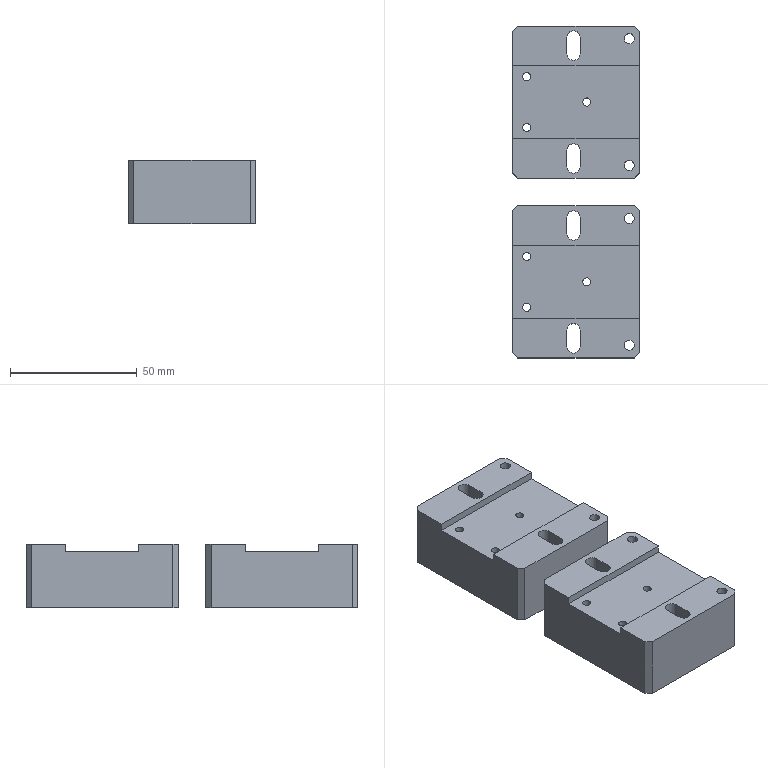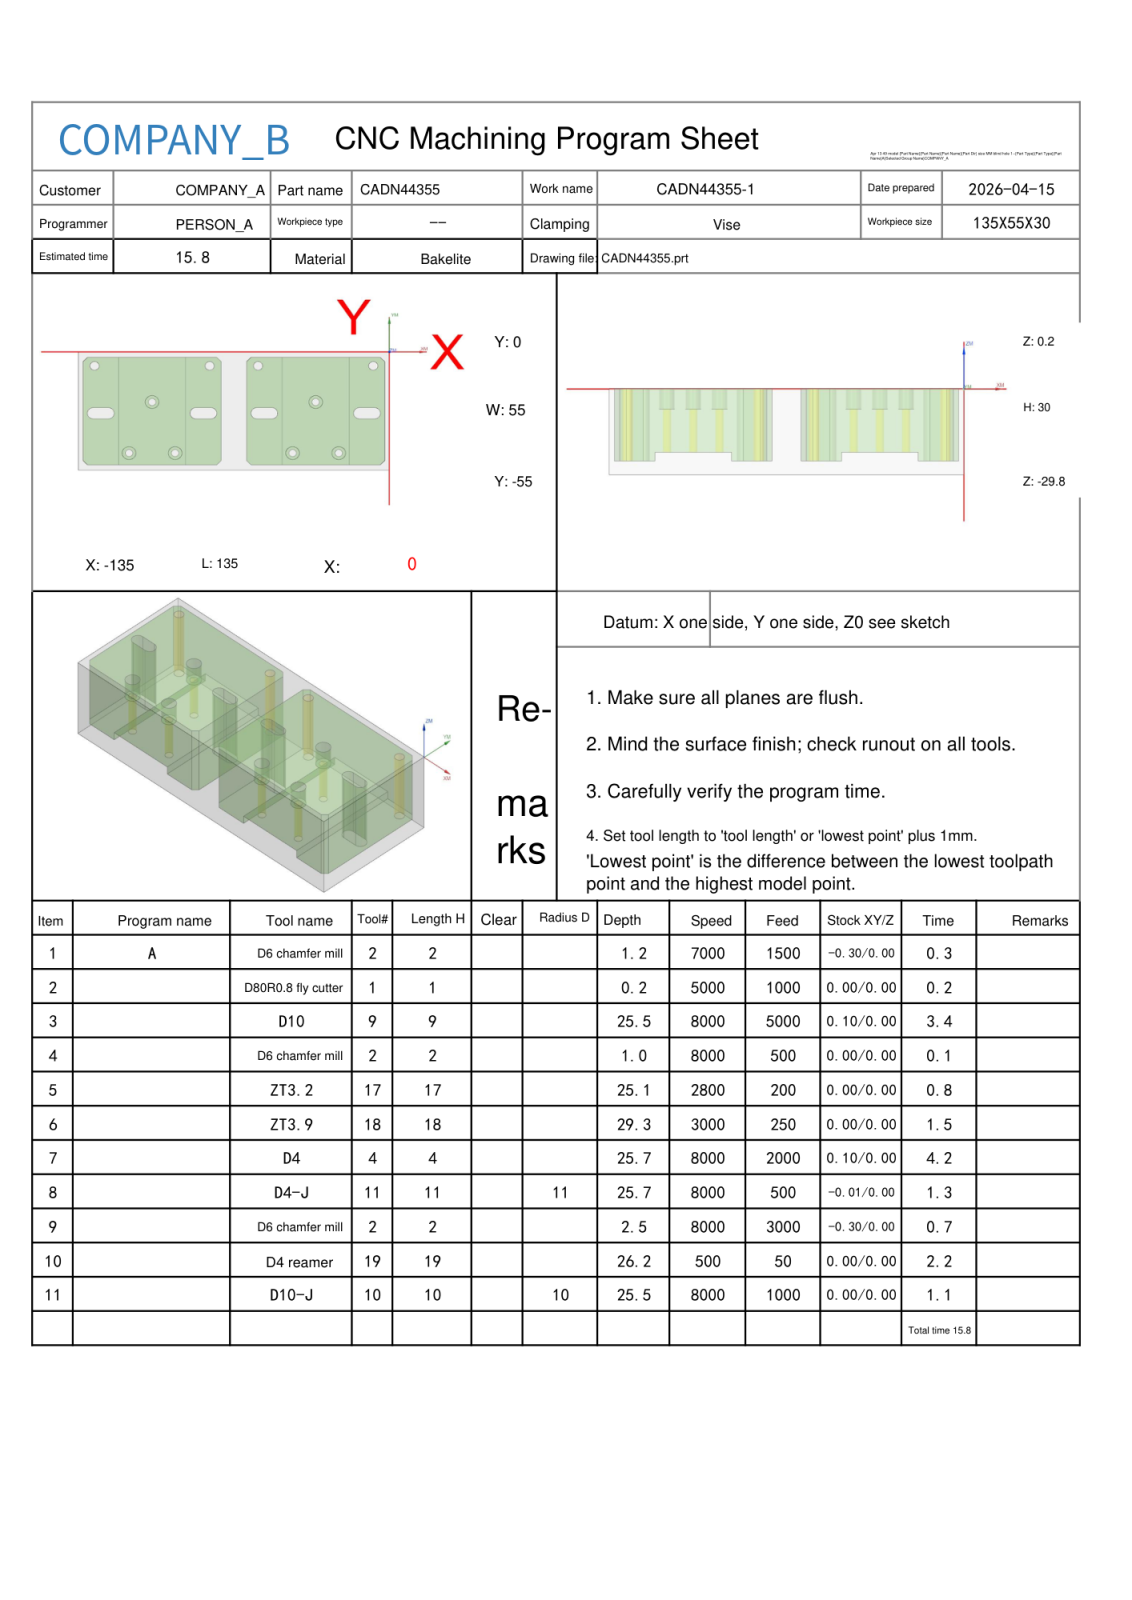NC program | NX | posted by the shop | part box 50 x 131 x 25 mm
Lines 1 to 1279 of 5183, first 1155 of 1277 lines:
%
O0001
(Machine time: 17.84 MIN)
(===Total Tool:9===)
(T2=D6 chamfer mill   D=6.   R=0.   D-  H02 Z=-2.3  )
(T1=D80R0.8 fly cutter D=80.  R=0.8  D-  H01 Z=0.    )
(T9=D10     D=10.  R=0.   D-  H09 Z=-25.3 )
(T17=ZT3.2  D=3.2  DR_a=120 D-  H17 Z=-24.92)
(T18=ZT3.9  D=3.9  DR_a=120 D-  H18 Z=-29.13)
(T4=D4      D=4.   R=0.   D-  H04 Z=-25.5 )
(T11=D4-J   D=4.   R=0.   D11 H11 Z=-25.5 )
(T19=D4 reamer   D=4.   DR_a=180 D-  H19 Z=-26.  )
(T10=D10-J  D=10.  R=0.   D10 H10 Z=-25.3 )
G80 G90 G17 G49 G40
G91 G28 Z0
M01
N1 T02 M06
(D6 chamfer mill  D=6. R=0. H=02 ce=-0.30 di=0.00)
G00 G90 G54 X-1.3 Y-41.546 M03 S7000
G43 H02 Z20.
M08
Z2.5
G01 Y-50.453 Z-.742 F1500.
X-1.338 Y-50.66 Z-.819
X-1.419 Y-50.855 Z-.895
X-1.538 Y-51.028 Z-.972
X-1.593 Y-51.083 Z-1.
X-3.417 Y-52.907
G02 X-4.124 Y-53.2 I-.707 J.707
G01 X-59.876
G02 X-60.583 Y-52.907 I0.0 J1.
G01 X-62.407 Y-51.083
G02 X-62.7 Y-50.376 I.707 J.707
G01 Y-4.624
G02 X-62.407 Y-3.917 I1. J0.0
G01 X-60.583 Y-2.093
G02 X-59.876 Y-1.8 I.707 J-.707
G01 X-4.124
G02 X-3.417 Y-2.093 I0.0 J-1.
G01 X-1.593 Y-3.917
G02 X-1.3 Y-4.624 I-.707 J-.707
G01 Y-50.376
G02 X-1.593 Y-51.083 I-1. J0.0
G01 X-1.946 Y-51.436
Z1.5
G00 Z20.
X-72.3 Y-41.546
Z2.5
G01 Y-50.453 Z-.742
X-72.338 Y-50.66 Z-.819
X-72.419 Y-50.855 Z-.895
X-72.538 Y-51.028 Z-.972
X-72.593 Y-51.083 Z-1.
X-74.417 Y-52.907
G02 X-75.124 Y-53.2 I-.707 J.707
G01 X-130.876
G02 X-131.583 Y-52.907 I0.0 J1.
G01 X-133.407 Y-51.083
G02 X-133.7 Y-50.376 I.707 J.707
G01 Y-4.624
G02 X-133.407 Y-3.917 I1. J0.0
G01 X-131.583 Y-2.093
G02 X-130.876 Y-1.8 I.707 J-.707
G01 X-75.124
G02 X-74.417 Y-2.093 I0.0 J-1.
G01 X-72.593 Y-3.917
G02 X-72.3 Y-4.624 I-.707 J-.707
G01 Y-50.376
G02 X-72.593 Y-51.083 I-1. J0.0
G01 X-72.946 Y-51.436
Z1.5
G00 Z20.
G91 G28 Z0.0
M05
M09
G91 G28 Z0.0
M01
N2 T01 M06
(D80R0.8 fly cutter  D=80. R=0.8 H=01 ce=0.00 di=0.00)
G00 G90 G54 X-178. Y-27.5 M03 S5000
G43 H01 Z20.
M08
Z2.
G01 Z0.0 F1000.
X-173.
X38.
X43.
Z2.
G00 Z20.
G91 G28 Z0.0
M05
M09
G91 G28 Z0.0
M01
N3 T09 M06
(D10  D=10. R=0. H=09 ce=0.10 di=0.00)
G00 G90 G54 X-32. Y-57.6 M03 S8000
G43 H09 Z20.
M08
Z.5
G01 X-60. Z.412 F5000.
G02 X-63.606 Y-56.106 Z.399 I0.0 J5.1
G01 X-65.606 Y-54.106 Z.39
G02 X-67.1 Y-50.5 Z.377 I3.606 J3.606
G01 Y-4.5 Z.232
G02 X-65.606 Y-.894 Z.219 I5.1 J0.0
G01 X-63.606 Y1.106 Z.21
G02 X-60. Y2.6 Z.198 I3.606 J-3.606
G01 X-4. Z.021
G02 X-.394 Y1.106 Z.008 I0.0 J-5.1
G01 X1.606 Y-.894 Z-.001
G02 X3.1 Y-4.5 Z-.014 I-3.606 J-3.606
G01 Y-50.5 Z-.159
G02 X1.606 Y-54.106 Z-.172 I-5.1 J0.0
G01 X-.394 Y-56.106 Z-.181
G02 X-4. Y-57.6 Z-.193 I-3.606 J3.606
G01 X-60. Z-.37
G02 X-63.606 Y-56.106 Z-.383 I0.0 J5.1
G01 X-65.606 Y-54.106 Z-.392
G02 X-67.1 Y-50.5 Z-.405 I3.606 J3.606
G01 Y-4.5 Z-.55
G02 X-65.606 Y-.894 Z-.563 I5.1 J0.0
G01 X-63.606 Y1.106 Z-.572
G02 X-60. Y2.6 Z-.584 I3.606 J-3.606
G01 X-4. Z-.761
G02 X-.394 Y1.106 Z-.774 I0.0 J-5.1
G01 X1.606 Y-.894 Z-.783
G02 X3.1 Y-4.5 Z-.795 I-3.606 J-3.606
G01 Y-50.5 Z-.941
G02 X1.606 Y-54.106 Z-.954 I-5.1 J0.0
G01 X-.394 Y-56.106 Z-.962
G02 X-4. Y-57.6 Z-.975 I-3.606 J3.606
G01 X-60. Z-1.152
G02 X-63.606 Y-56.106 Z-1.165 I0.0 J5.1
G01 X-65.606 Y-54.106 Z-1.174
G02 X-67.1 Y-50.5 Z-1.186 I3.606 J3.606
G01 Y-4.5 Z-1.332
G02 X-65.606 Y-.894 Z-1.344 I5.1 J0.0
G01 X-63.606 Y1.106 Z-1.353
G02 X-60. Y2.6 Z-1.366 I3.606 J-3.606
G01 X-4. Z-1.543
G02 X-.394 Y1.106 Z-1.556 I0.0 J-5.1
G01 X1.606 Y-.894 Z-1.565
G02 X3.1 Y-4.5 Z-1.577 I-3.606 J-3.606
G01 Y-50.5 Z-1.723
G02 X1.606 Y-54.106 Z-1.735 I-5.1 J0.0
G01 X-.394 Y-56.106 Z-1.744
G02 X-4. Y-57.6 Z-1.757 I-3.606 J3.606
G01 X-60. Z-1.934
G02 X-63.606 Y-56.106 Z-1.947 I0.0 J5.1
G01 X-65.606 Y-54.106 Z-1.956
G02 X-67.1 Y-50.5 Z-1.968 I3.606 J3.606
G01 Y-4.5 Z-2.114
G02 X-65.606 Y-.894 Z-2.126 I5.1 J0.0
G01 X-63.606 Y1.106 Z-2.135
G02 X-60. Y2.6 Z-2.148 I3.606 J-3.606
G01 X-4. Z-2.325
G02 X-.394 Y1.106 Z-2.338 I0.0 J-5.1
G01 X1.606 Y-.894 Z-2.346
G02 X3.1 Y-4.5 Z-2.359 I-3.606 J-3.606
G01 Y-50.5 Z-2.505
G02 X1.606 Y-54.106 Z-2.517 I-5.1 J0.0
G01 X-.394 Y-56.106 Z-2.526
G02 X-4. Y-57.6 Z-2.539 I-3.606 J3.606
G01 X-60. Z-2.716
G02 X-63.606 Y-56.106 Z-2.728 I0.0 J5.1
G01 X-65.606 Y-54.106 Z-2.737
G02 X-67.1 Y-50.5 Z-2.75 I3.606 J3.606
G01 Y-4.5 Z-2.895
G02 X-65.606 Y-.894 Z-2.908 I5.1 J0.0
G01 X-63.606 Y1.106 Z-2.917
G02 X-60. Y2.6 Z-2.93 I3.606 J-3.606
G01 X-4. Z-3.107
G02 X-.394 Y1.106 Z-3.119 I0.0 J-5.1
G01 X1.606 Y-.894 Z-3.128
G02 X3.1 Y-4.5 Z-3.141 I-3.606 J-3.606
G01 Y-50.5 Z-3.286
G02 X1.606 Y-54.106 Z-3.299 I-5.1 J0.0
G01 X-.394 Y-56.106 Z-3.308
G02 X-4. Y-57.6 Z-3.321 I-3.606 J3.606
G01 X-60. Z-3.498
G02 X-63.606 Y-56.106 Z-3.51 I0.0 J5.1
G01 X-65.606 Y-54.106 Z-3.519
G02 X-67.1 Y-50.5 Z-3.532 I3.606 J3.606
G01 Y-4.5 Z-3.677
G02 X-65.606 Y-.894 Z-3.69 I5.1 J0.0
G01 X-63.606 Y1.106 Z-3.699
G02 X-60. Y2.6 Z-3.712 I3.606 J-3.606
G01 X-4. Z-3.888
G02 X-.394 Y1.106 Z-3.901 I0.0 J-5.1
G01 X1.606 Y-.894 Z-3.91
G02 X3.1 Y-4.5 Z-3.923 I-3.606 J-3.606
G01 Y-50.5 Z-4.068
G02 X1.606 Y-54.106 Z-4.081 I-5.1 J0.0
G01 X-.394 Y-56.106 Z-4.09
G02 X-4. Y-57.6 Z-4.102 I-3.606 J3.606
G01 X-60. Z-4.279
G02 X-63.606 Y-56.106 Z-4.292 I0.0 J5.1
G01 X-65.606 Y-54.106 Z-4.301
G02 X-67.1 Y-50.5 Z-4.314 I3.606 J3.606
G01 Y-4.5 Z-4.459
G02 X-65.606 Y-.894 Z-4.472 I5.1 J0.0
G01 X-63.606 Y1.106 Z-4.481
G02 X-60. Y2.6 Z-4.493 I3.606 J-3.606
G01 X-4. Z-4.67
G02 X-.394 Y1.106 Z-4.683 I0.0 J-5.1
G01 X1.606 Y-.894 Z-4.692
G02 X3.1 Y-4.5 Z-4.705 I-3.606 J-3.606
G01 Y-50.5 Z-4.85
G02 X1.606 Y-54.106 Z-4.863 I-5.1 J0.0
G01 X-.394 Y-56.106 Z-4.872
G02 X-4. Y-57.6 Z-4.884 I-3.606 J3.606
G01 X-60. Z-5.061
G02 X-63.606 Y-56.106 Z-5.074 I0.0 J5.1
G01 X-65.606 Y-54.106 Z-5.083
G02 X-67.1 Y-50.5 Z-5.095 I3.606 J3.606
G01 Y-4.5 Z-5.241
G02 X-65.606 Y-.894 Z-5.254 I5.1 J0.0
G01 X-63.606 Y1.106 Z-5.262
G02 X-60. Y2.6 Z-5.275 I3.606 J-3.606
G01 X-4. Z-5.452
G02 X-.394 Y1.106 Z-5.465 I0.0 J-5.1
G01 X1.606 Y-.894 Z-5.474
G02 X3.1 Y-4.5 Z-5.486 I-3.606 J-3.606
G01 Y-50.5 Z-5.632
G02 X1.606 Y-54.106 Z-5.644 I-5.1 J0.0
G01 X-.394 Y-56.106 Z-5.653
G02 X-4. Y-57.6 Z-5.666 I-3.606 J3.606
G01 X-60. Z-5.843
G02 X-63.606 Y-56.106 Z-5.856 I0.0 J5.1
G01 X-65.606 Y-54.106 Z-5.865
G02 X-67.1 Y-50.5 Z-5.877 I3.606 J3.606
G01 Y-4.5 Z-6.023
G02 X-65.606 Y-.894 Z-6.035 I5.1 J0.0
G01 X-63.606 Y1.106 Z-6.044
G02 X-60. Y2.6 Z-6.057 I3.606 J-3.606
G01 X-4. Z-6.234
G02 X-.394 Y1.106 Z-6.247 I0.0 J-5.1
G01 X1.606 Y-.894 Z-6.256
G02 X3.1 Y-4.5 Z-6.268 I-3.606 J-3.606
G01 Y-50.5 Z-6.414
G02 X1.606 Y-54.106 Z-6.426 I-5.1 J0.0
G01 X-.394 Y-56.106 Z-6.435
G02 X-4. Y-57.6 Z-6.448 I-3.606 J3.606
G01 X-60. Z-6.625
G02 X-63.606 Y-56.106 Z-6.638 I0.0 J5.1
G01 X-65.606 Y-54.106 Z-6.646
G02 X-67.1 Y-50.5 Z-6.659 I3.606 J3.606
G01 Y-4.5 Z-6.805
G02 X-65.606 Y-.894 Z-6.817 I5.1 J0.0
G01 X-63.606 Y1.106 Z-6.826
G02 X-60. Y2.6 Z-6.839 I3.606 J-3.606
G01 X-4. Z-7.016
G02 X-.394 Y1.106 Z-7.028 I0.0 J-5.1
G01 X1.606 Y-.894 Z-7.037
G02 X3.1 Y-4.5 Z-7.05 I-3.606 J-3.606
G01 Y-50.5 Z-7.195
G02 X1.606 Y-54.106 Z-7.208 I-5.1 J0.0
G01 X-.394 Y-56.106 Z-7.217
G02 X-4. Y-57.6 Z-7.23 I-3.606 J3.606
G01 X-60. Z-7.407
G02 X-63.606 Y-56.106 Z-7.419 I0.0 J5.1
G01 X-65.606 Y-54.106 Z-7.428
G02 X-67.1 Y-50.5 Z-7.441 I3.606 J3.606
G01 Y-4.5 Z-7.586
G02 X-65.606 Y-.894 Z-7.599 I5.1 J0.0
G01 X-63.606 Y1.106 Z-7.608
G02 X-60. Y2.6 Z-7.621 I3.606 J-3.606
G01 X-4. Z-7.798
G02 X-.394 Y1.106 Z-7.81 I0.0 J-5.1
G01 X1.606 Y-.894 Z-7.819
G02 X3.1 Y-4.5 Z-7.832 I-3.606 J-3.606
G01 Y-50.5 Z-7.977
G02 X1.606 Y-54.106 Z-7.99 I-5.1 J0.0
G01 X-.394 Y-56.106 Z-7.999
G02 X-4. Y-57.6 Z-8.012 I-3.606 J3.606
G01 X-60. Z-8.188
G02 X-63.606 Y-56.106 Z-8.201 I0.0 J5.1
G01 X-65.606 Y-54.106 Z-8.21
G02 X-67.1 Y-50.5 Z-8.223 I3.606 J3.606
G01 Y-4.5 Z-8.368
G02 X-65.606 Y-.894 Z-8.381 I5.1 J0.0
G01 X-63.606 Y1.106 Z-8.39
G02 X-60. Y2.6 Z-8.402 I3.606 J-3.606
G01 X-4. Z-8.579
G02 X-.394 Y1.106 Z-8.592 I0.0 J-5.1
G01 X1.606 Y-.894 Z-8.601
G02 X3.1 Y-4.5 Z-8.614 I-3.606 J-3.606
G01 Y-50.5 Z-8.759
G02 X1.606 Y-54.106 Z-8.772 I-5.1 J0.0
G01 X-.394 Y-56.106 Z-8.781
G02 X-4. Y-57.6 Z-8.793 I-3.606 J3.606
G01 X-60. Z-8.97
G02 X-63.606 Y-56.106 Z-8.983 I0.0 J5.1
G01 X-65.606 Y-54.106 Z-8.992
G02 X-67.1 Y-50.5 Z-9.005 I3.606 J3.606
G01 Y-4.5 Z-9.15
G02 X-65.606 Y-.894 Z-9.163 I5.1 J0.0
G01 X-63.606 Y1.106 Z-9.172
G02 X-60. Y2.6 Z-9.184 I3.606 J-3.606
G01 X-4. Z-9.361
G02 X-.394 Y1.106 Z-9.374 I0.0 J-5.1
G01 X1.606 Y-.894 Z-9.383
G02 X3.1 Y-4.5 Z-9.395 I-3.606 J-3.606
G01 Y-50.5 Z-9.541
G02 X1.606 Y-54.106 Z-9.554 I-5.1 J0.0
G01 X-.394 Y-56.106 Z-9.562
G02 X-4. Y-57.6 Z-9.575 I-3.606 J3.606
G01 X-60. Z-9.752
G02 X-63.606 Y-56.106 Z-9.765 I0.0 J5.1
G01 X-65.606 Y-54.106 Z-9.774
G02 X-67.1 Y-50.5 Z-9.786 I3.606 J3.606
G01 Y-4.5 Z-9.932
G02 X-65.606 Y-.894 Z-9.944 I5.1 J0.0
G01 X-63.606 Y1.106 Z-9.953
G02 X-60. Y2.6 Z-9.966 I3.606 J-3.606
G01 X-4. Z-10.143
G02 X-.394 Y1.106 Z-10.156 I0.0 J-5.1
G01 X1.606 Y-.894 Z-10.165
G02 X3.1 Y-4.5 Z-10.177 I-3.606 J-3.606
G01 Y-50.5 Z-10.323
G02 X1.606 Y-54.106 Z-10.335 I-5.1 J0.0
G01 X-.394 Y-56.106 Z-10.344
G02 X-4. Y-57.6 Z-10.357 I-3.606 J3.606
G01 X-60. Z-10.534
G02 X-63.606 Y-56.106 Z-10.547 I0.0 J5.1
G01 X-65.606 Y-54.106 Z-10.556
G02 X-67.1 Y-50.5 Z-10.568 I3.606 J3.606
G01 Y-4.5 Z-10.714
G02 X-65.606 Y-.894 Z-10.726 I5.1 J0.0
G01 X-63.606 Y1.106 Z-10.735
G02 X-60. Y2.6 Z-10.748 I3.606 J-3.606
G01 X-4. Z-10.925
G02 X-.394 Y1.106 Z-10.938 I0.0 J-5.1
G01 X1.606 Y-.894 Z-10.946
G02 X3.1 Y-4.5 Z-10.959 I-3.606 J-3.606
G01 Y-50.5 Z-11.105
G02 X1.606 Y-54.106 Z-11.117 I-5.1 J0.0
G01 X-.394 Y-56.106 Z-11.126
G02 X-4. Y-57.6 Z-11.139 I-3.606 J3.606
G01 X-60. Z-11.316
G02 X-63.606 Y-56.106 Z-11.328 I0.0 J5.1
G01 X-65.606 Y-54.106 Z-11.337
G02 X-67.1 Y-50.5 Z-11.35 I3.606 J3.606
G01 Y-4.5 Z-11.495
G02 X-65.606 Y-.894 Z-11.508 I5.1 J0.0
G01 X-63.606 Y1.106 Z-11.517
G02 X-60. Y2.6 Z-11.53 I3.606 J-3.606
G01 X-4. Z-11.707
G02 X-.394 Y1.106 Z-11.719 I0.0 J-5.1
G01 X1.606 Y-.894 Z-11.728
G02 X3.1 Y-4.5 Z-11.741 I-3.606 J-3.606
G01 Y-50.5 Z-11.886
G02 X1.606 Y-54.106 Z-11.899 I-5.1 J0.0
G01 X-.394 Y-56.106 Z-11.908
G02 X-4. Y-57.6 Z-11.921 I-3.606 J3.606
G01 X-60. Z-12.098
G02 X-63.606 Y-56.106 Z-12.11 I0.0 J5.1
G01 X-65.606 Y-54.106 Z-12.119
G02 X-67.1 Y-50.5 Z-12.132 I3.606 J3.606
G01 Y-4.5 Z-12.277
G02 X-65.606 Y-.894 Z-12.29 I5.1 J0.0
G01 X-63.606 Y1.106 Z-12.299
G02 X-60. Y2.6 Z-12.312 I3.606 J-3.606
G01 X-4. Z-12.488
G02 X-.394 Y1.106 Z-12.501 I0.0 J-5.1
G01 X1.606 Y-.894 Z-12.51
G02 X3.1 Y-4.5 Z-12.523 I-3.606 J-3.606
G01 Y-50.5 Z-12.668
G02 X1.606 Y-54.106 Z-12.681 I-5.1 J0.0
G01 X-.394 Y-56.106 Z-12.69
G02 X-4. Y-57.6 Z-12.702 I-3.606 J3.606
G01 X-60. Z-12.879
G02 X-63.606 Y-56.106 Z-12.892 I0.0 J5.1
G01 X-65.606 Y-54.106 Z-12.901
G02 X-67.1 Y-50.5 Z-12.914 I3.606 J3.606
G01 Y-4.5 Z-13.059
G02 X-65.606 Y-.894 Z-13.072 I5.1 J0.0
G01 X-63.606 Y1.106 Z-13.081
G02 X-60. Y2.6 Z-13.093 I3.606 J-3.606
G01 X-4. Z-13.27
G02 X-.394 Y1.106 Z-13.283 I0.0 J-5.1
G01 X1.606 Y-.894 Z-13.292
G02 X3.1 Y-4.5 Z-13.305 I-3.606 J-3.606
G01 Y-50.5 Z-13.45
G02 X1.606 Y-54.106 Z-13.463 I-5.1 J0.0
G01 X-.394 Y-56.106 Z-13.472
G02 X-4. Y-57.6 Z-13.484 I-3.606 J3.606
G01 X-60. Z-13.661
G02 X-63.606 Y-56.106 Z-13.674 I0.0 J5.1
G01 X-65.606 Y-54.106 Z-13.683
G02 X-67.1 Y-50.5 Z-13.695 I3.606 J3.606
G01 Y-4.5 Z-13.841
G02 X-65.606 Y-.894 Z-13.854 I5.1 J0.0
G01 X-63.606 Y1.106 Z-13.862
G02 X-60. Y2.6 Z-13.875 I3.606 J-3.606
G01 X-4. Z-14.052
G02 X-.394 Y1.106 Z-14.065 I0.0 J-5.1
G01 X1.606 Y-.894 Z-14.074
G02 X3.1 Y-4.5 Z-14.086 I-3.606 J-3.606
G01 Y-50.5 Z-14.232
G02 X1.606 Y-54.106 Z-14.244 I-5.1 J0.0
G01 X-.394 Y-56.106 Z-14.253
G02 X-4. Y-57.6 Z-14.266 I-3.606 J3.606
G01 X-60. Z-14.443
G02 X-63.606 Y-56.106 Z-14.456 I0.0 J5.1
G01 X-65.606 Y-54.106 Z-14.465
G02 X-67.1 Y-50.5 Z-14.477 I3.606 J3.606
G01 Y-4.5 Z-14.623
G02 X-65.606 Y-.894 Z-14.635 I5.1 J0.0
G01 X-63.606 Y1.106 Z-14.644
G02 X-60. Y2.6 Z-14.657 I3.606 J-3.606
G01 X-4. Z-14.834
G02 X-.394 Y1.106 Z-14.847 I0.0 J-5.1
G01 X1.606 Y-.894 Z-14.856
G02 X3.1 Y-4.5 Z-14.868 I-3.606 J-3.606
G01 Y-50.5 Z-15.014
G02 X1.606 Y-54.106 Z-15.026 I-5.1 J0.0
G01 X-.394 Y-56.106 Z-15.035
G02 X-4. Y-57.6 Z-15.048 I-3.606 J3.606
G01 X-60. Z-15.225
G02 X-63.606 Y-56.106 Z-15.238 I0.0 J5.1
G01 X-65.606 Y-54.106 Z-15.246
G02 X-67.1 Y-50.5 Z-15.259 I3.606 J3.606
G01 Y-4.5 Z-15.405
G02 X-65.606 Y-.894 Z-15.417 I5.1 J0.0
G01 X-63.606 Y1.106 Z-15.426
G02 X-60. Y2.6 Z-15.439 I3.606 J-3.606
G01 X-4. Z-15.616
G02 X-.394 Y1.106 Z-15.628 I0.0 J-5.1
G01 X1.606 Y-.894 Z-15.637
G02 X3.1 Y-4.5 Z-15.65 I-3.606 J-3.606
G01 Y-50.5 Z-15.795
G02 X1.606 Y-54.106 Z-15.808 I-5.1 J0.0
G01 X-.394 Y-56.106 Z-15.817
G02 X-4. Y-57.6 Z-15.83 I-3.606 J3.606
G01 X-60. Z-16.007
G02 X-63.606 Y-56.106 Z-16.019 I0.0 J5.1
G01 X-65.606 Y-54.106 Z-16.028
G02 X-67.1 Y-50.5 Z-16.041 I3.606 J3.606
G01 Y-4.5 Z-16.186
G02 X-65.606 Y-.894 Z-16.199 I5.1 J0.0
G01 X-63.606 Y1.106 Z-16.208
G02 X-60. Y2.6 Z-16.221 I3.606 J-3.606
G01 X-4. Z-16.398
G02 X-.394 Y1.106 Z-16.41 I0.0 J-5.1
G01 X1.606 Y-.894 Z-16.419
G02 X3.1 Y-4.5 Z-16.432 I-3.606 J-3.606
G01 Y-50.5 Z-16.577
G02 X1.606 Y-54.106 Z-16.59 I-5.1 J0.0
G01 X-.394 Y-56.106 Z-16.599
G02 X-4. Y-57.6 Z-16.612 I-3.606 J3.606
G01 X-60. Z-16.788
G02 X-63.606 Y-56.106 Z-16.801 I0.0 J5.1
G01 X-65.606 Y-54.106 Z-16.81
G02 X-67.1 Y-50.5 Z-16.823 I3.606 J3.606
G01 Y-4.5 Z-16.968
G02 X-65.606 Y-.894 Z-16.981 I5.1 J0.0
G01 X-63.606 Y1.106 Z-16.99
G02 X-60. Y2.6 Z-17.002 I3.606 J-3.606
G01 X-4. Z-17.179
G02 X-.394 Y1.106 Z-17.192 I0.0 J-5.1
G01 X1.606 Y-.894 Z-17.201
G02 X3.1 Y-4.5 Z-17.214 I-3.606 J-3.606
G01 Y-50.5 Z-17.359
G02 X1.606 Y-54.106 Z-17.372 I-5.1 J0.0
G01 X-.394 Y-56.106 Z-17.381
G02 X-4. Y-57.6 Z-17.393 I-3.606 J3.606
G01 X-60. Z-17.57
G02 X-63.606 Y-56.106 Z-17.583 I0.0 J5.1
G01 X-65.606 Y-54.106 Z-17.592
G02 X-67.1 Y-50.5 Z-17.605 I3.606 J3.606
G01 Y-4.5 Z-17.75
G02 X-65.606 Y-.894 Z-17.763 I5.1 J0.0
G01 X-63.606 Y1.106 Z-17.772
G02 X-60. Y2.6 Z-17.784 I3.606 J-3.606
G01 X-4. Z-17.961
G02 X-.394 Y1.106 Z-17.974 I0.0 J-5.1
G01 X1.606 Y-.894 Z-17.983
G02 X3.1 Y-4.5 Z-17.995 I-3.606 J-3.606
G01 Y-50.5 Z-18.141
G02 X1.606 Y-54.106 Z-18.154 I-5.1 J0.0
G01 X-.394 Y-56.106 Z-18.162
G02 X-4. Y-57.6 Z-18.175 I-3.606 J3.606
G01 X-60. Z-18.352
G02 X-63.606 Y-56.106 Z-18.365 I0.0 J5.1
G01 X-65.606 Y-54.106 Z-18.374
G02 X-67.1 Y-50.5 Z-18.386 I3.606 J3.606
G01 Y-4.5 Z-18.532
G02 X-65.606 Y-.894 Z-18.544 I5.1 J0.0
G01 X-63.606 Y1.106 Z-18.553
G02 X-60. Y2.6 Z-18.566 I3.606 J-3.606
G01 X-4. Z-18.743
G02 X-.394 Y1.106 Z-18.756 I0.0 J-5.1
G01 X1.606 Y-.894 Z-18.765
G02 X3.1 Y-4.5 Z-18.777 I-3.606 J-3.606
G01 Y-50.5 Z-18.923
G02 X1.606 Y-54.106 Z-18.935 I-5.1 J0.0
G01 X-.394 Y-56.106 Z-18.944
G02 X-4. Y-57.6 Z-18.957 I-3.606 J3.606
G01 X-60. Z-19.134
G02 X-63.606 Y-56.106 Z-19.147 I0.0 J5.1
G01 X-65.606 Y-54.106 Z-19.156
G02 X-67.1 Y-50.5 Z-19.168 I3.606 J3.606
G01 Y-4.5 Z-19.314
G02 X-65.606 Y-.894 Z-19.326 I5.1 J0.0
G01 X-63.606 Y1.106 Z-19.335
G02 X-60. Y2.6 Z-19.348 I3.606 J-3.606
G01 X-4. Z-19.525
G02 X-.394 Y1.106 Z-19.538 I0.0 J-5.1
G01 X1.606 Y-.894 Z-19.546
G02 X3.1 Y-4.5 Z-19.559 I-3.606 J-3.606
G01 Y-50.5 Z-19.705
G02 X1.606 Y-54.106 Z-19.717 I-5.1 J0.0
G01 X-.394 Y-56.106 Z-19.726
G02 X-4. Y-57.6 Z-19.739 I-3.606 J3.606
G01 X-60. Z-19.916
G02 X-63.606 Y-56.106 Z-19.928 I0.0 J5.1
G01 X-65.606 Y-54.106 Z-19.937
G02 X-67.1 Y-50.5 Z-19.95 I3.606 J3.606
G01 Y-4.5 Z-20.095
G02 X-65.606 Y-.894 Z-20.108 I5.1 J0.0
G01 X-63.606 Y1.106 Z-20.117
G02 X-60. Y2.6 Z-20.13 I3.606 J-3.606
G01 X-4. Z-20.307
G02 X-.394 Y1.106 Z-20.319 I0.0 J-5.1
G01 X1.606 Y-.894 Z-20.328
G02 X3.1 Y-4.5 Z-20.341 I-3.606 J-3.606
G01 Y-50.5 Z-20.486
G02 X1.606 Y-54.106 Z-20.499 I-5.1 J0.0
G01 X-.394 Y-56.106 Z-20.508
G02 X-4. Y-57.6 Z-20.521 I-3.606 J3.606
G01 X-60. Z-20.698
G02 X-63.606 Y-56.106 Z-20.71 I0.0 J5.1
G01 X-65.606 Y-54.106 Z-20.719
G02 X-67.1 Y-50.5 Z-20.732 I3.606 J3.606
G01 Y-4.5 Z-20.877
G02 X-65.606 Y-.894 Z-20.89 I5.1 J0.0
G01 X-63.606 Y1.106 Z-20.899
G02 X-60. Y2.6 Z-20.912 I3.606 J-3.606
G01 X-4. Z-21.088
G02 X-.394 Y1.106 Z-21.101 I0.0 J-5.1
G01 X1.606 Y-.894 Z-21.11
G02 X3.1 Y-4.5 Z-21.123 I-3.606 J-3.606
G01 Y-50.5 Z-21.268
G02 X1.606 Y-54.106 Z-21.281 I-5.1 J0.0
G01 X-.394 Y-56.106 Z-21.29
G02 X-4. Y-57.6 Z-21.302 I-3.606 J3.606
G01 X-60. Z-21.479
G02 X-63.606 Y-56.106 Z-21.492 I0.0 J5.1
G01 X-65.606 Y-54.106 Z-21.501
G02 X-67.1 Y-50.5 Z-21.514 I3.606 J3.606
G01 Y-4.5 Z-21.659
G02 X-65.606 Y-.894 Z-21.672 I5.1 J0.0
G01 X-63.606 Y1.106 Z-21.681
G02 X-60. Y2.6 Z-21.693 I3.606 J-3.606
G01 X-4. Z-21.87
G02 X-.394 Y1.106 Z-21.883 I0.0 J-5.1
G01 X1.606 Y-.894 Z-21.892
G02 X3.1 Y-4.5 Z-21.905 I-3.606 J-3.606
G01 Y-50.5 Z-22.05
G02 X1.606 Y-54.106 Z-22.063 I-5.1 J0.0
G01 X-.394 Y-56.106 Z-22.072
G02 X-4. Y-57.6 Z-22.084 I-3.606 J3.606
G01 X-60. Z-22.261
G02 X-63.606 Y-56.106 Z-22.274 I0.0 J5.1
G01 X-65.606 Y-54.106 Z-22.283
G02 X-67.1 Y-50.5 Z-22.295 I3.606 J3.606
G01 Y-4.5 Z-22.441
G02 X-65.606 Y-.894 Z-22.454 I5.1 J0.0
G01 X-63.606 Y1.106 Z-22.462
G02 X-60. Y2.6 Z-22.475 I3.606 J-3.606
G01 X-4. Z-22.652
G02 X-.394 Y1.106 Z-22.665 I0.0 J-5.1
G01 X1.606 Y-.894 Z-22.674
G02 X3.1 Y-4.5 Z-22.686 I-3.606 J-3.606
G01 Y-50.5 Z-22.832
G02 X1.606 Y-54.106 Z-22.844 I-5.1 J0.0
G01 X-.394 Y-56.106 Z-22.853
G02 X-4. Y-57.6 Z-22.866 I-3.606 J3.606
G01 X-60. Z-23.043
G02 X-63.606 Y-56.106 Z-23.056 I0.0 J5.1
G01 X-65.606 Y-54.106 Z-23.065
G02 X-67.1 Y-50.5 Z-23.077 I3.606 J3.606
G01 Y-4.5 Z-23.223
G02 X-65.606 Y-.894 Z-23.235 I5.1 J0.0
G01 X-63.606 Y1.106 Z-23.244
G02 X-60. Y2.6 Z-23.257 I3.606 J-3.606
G01 X-4. Z-23.434
G02 X-.394 Y1.106 Z-23.447 I0.0 J-5.1
G01 X1.606 Y-.894 Z-23.456
G02 X3.1 Y-4.5 Z-23.468 I-3.606 J-3.606
G01 Y-50.5 Z-23.614
G02 X1.606 Y-54.106 Z-23.626 I-5.1 J0.0
G01 X-.394 Y-56.106 Z-23.635
G02 X-4. Y-57.6 Z-23.648 I-3.606 J3.606
G01 X-60. Z-23.825
G02 X-63.606 Y-56.106 Z-23.838 I0.0 J5.1
G01 X-65.606 Y-54.106 Z-23.846
G02 X-67.1 Y-50.5 Z-23.859 I3.606 J3.606
G01 Y-4.5 Z-24.005
G02 X-65.606 Y-.894 Z-24.017 I5.1 J0.0
G01 X-63.606 Y1.106 Z-24.026
G02 X-60. Y2.6 Z-24.039 I3.606 J-3.606
G01 X-4. Z-24.216
G02 X-.394 Y1.106 Z-24.228 I0.0 J-5.1
G01 X1.606 Y-.894 Z-24.237
G02 X3.1 Y-4.5 Z-24.25 I-3.606 J-3.606
G01 Y-50.5 Z-24.395
G02 X1.606 Y-54.106 Z-24.408 I-5.1 J0.0
G01 X-.394 Y-56.106 Z-24.417
G02 X-4. Y-57.6 Z-24.43 I-3.606 J3.606
G01 X-60. Z-24.607
G02 X-63.606 Y-56.106 Z-24.619 I0.0 J5.1
G01 X-65.606 Y-54.106 Z-24.628
G02 X-67.1 Y-50.5 Z-24.641 I3.606 J3.606
G01 Y-4.5 Z-24.786
G02 X-65.606 Y-.894 Z-24.799 I5.1 J0.0
G01 X-63.606 Y1.106 Z-24.808
G02 X-60. Y2.6 Z-24.821 I3.606 J-3.606
G01 X-4. Z-24.998
G02 X-.394 Y1.106 Z-25.01 I0.0 J-5.1
G01 X1.606 Y-.894 Z-25.019
G02 X3.1 Y-4.5 Z-25.032 I-3.606 J-3.606
G01 Y-50.5 Z-25.177
G02 X1.606 Y-54.106 Z-25.19 I-5.1 J0.0
G01 X-.394 Y-56.106 Z-25.199
G02 X-4. Y-57.6 Z-25.212 I-3.606 J3.606
G01 X-32. Z-25.3
X-60.
G02 X-63.606 Y-56.106 I0.0 J5.1
G01 X-65.606 Y-54.106
G02 X-67.1 Y-50.5 I3.606 J3.606
G01 Y-4.5
G02 X-65.606 Y-.894 I5.1 J0.0
G01 X-63.606 Y1.106
G02 X-60. Y2.6 I3.606 J-3.606
G01 X-4.
G02 X-.394 Y1.106 I0.0 J-5.1
G01 X1.606 Y-.894
G02 X3.1 Y-4.5 I-3.606 J-3.606
G01 Y-50.5
G02 X1.606 Y-54.106 I-5.1 J0.0
G01 X-.394 Y-56.106
G02 X-4. Y-57.6 I-3.606 J3.606
G01 X-32.
X-32.5
Z-24.3
G00 Z20.
X-103.
Z.5
G01 X-131. Z.412
G02 X-134.606 Y-56.106 Z.399 I0.0 J5.1
G01 X-136.606 Y-54.106 Z.39
G02 X-138.1 Y-50.5 Z.377 I3.606 J3.606
G01 Y-4.5 Z.232
G02 X-136.606 Y-.894 Z.219 I5.1 J0.0
G01 X-134.606 Y1.106 Z.21
G02 X-131. Y2.6 Z.198 I3.606 J-3.606
G01 X-75. Z.021
G02 X-71.394 Y1.106 Z.008 I0.0 J-5.1
G01 X-69.394 Y-.894 Z-.001
G02 X-67.9 Y-4.5 Z-.014 I-3.606 J-3.606
G01 Y-50.5 Z-.159
G02 X-69.394 Y-54.106 Z-.172 I-5.1 J0.0
G01 X-71.394 Y-56.106 Z-.181
G02 X-75. Y-57.6 Z-.193 I-3.606 J3.606
G01 X-131. Z-.37
G02 X-134.606 Y-56.106 Z-.383 I0.0 J5.1
G01 X-136.606 Y-54.106 Z-.392
G02 X-138.1 Y-50.5 Z-.405 I3.606 J3.606
G01 Y-4.5 Z-.55
G02 X-136.606 Y-.894 Z-.563 I5.1 J0.0
G01 X-134.606 Y1.106 Z-.572
G02 X-131. Y2.6 Z-.584 I3.606 J-3.606
G01 X-75. Z-.761
G02 X-71.394 Y1.106 Z-.774 I0.0 J-5.1
G01 X-69.394 Y-.894 Z-.783
G02 X-67.9 Y-4.5 Z-.795 I-3.606 J-3.606
G01 Y-50.5 Z-.941
G02 X-69.394 Y-54.106 Z-.954 I-5.1 J0.0
G01 X-71.394 Y-56.106 Z-.962
G02 X-75. Y-57.6 Z-.975 I-3.606 J3.606
G01 X-131. Z-1.152
G02 X-134.606 Y-56.106 Z-1.165 I0.0 J5.1
G01 X-136.606 Y-54.106 Z-1.174
G02 X-138.1 Y-50.5 Z-1.186 I3.606 J3.606
G01 Y-4.5 Z-1.332
G02 X-136.606 Y-.894 Z-1.344 I5.1 J0.0
G01 X-134.606 Y1.106 Z-1.353
G02 X-131. Y2.6 Z-1.366 I3.606 J-3.606
G01 X-75. Z-1.543
G02 X-71.394 Y1.106 Z-1.556 I0.0 J-5.1
G01 X-69.394 Y-.894 Z-1.565
G02 X-67.9 Y-4.5 Z-1.577 I-3.606 J-3.606
G01 Y-50.5 Z-1.723
G02 X-69.394 Y-54.106 Z-1.735 I-5.1 J0.0
G01 X-71.394 Y-56.106 Z-1.744
G02 X-75. Y-57.6 Z-1.757 I-3.606 J3.606
G01 X-131. Z-1.934
G02 X-134.606 Y-56.106 Z-1.947 I0.0 J5.1
G01 X-136.606 Y-54.106 Z-1.956
G02 X-138.1 Y-50.5 Z-1.968 I3.606 J3.606
G01 Y-4.5 Z-2.114
G02 X-136.606 Y-.894 Z-2.126 I5.1 J0.0
G01 X-134.606 Y1.106 Z-2.135
G02 X-131. Y2.6 Z-2.148 I3.606 J-3.606
G01 X-75. Z-2.325
G02 X-71.394 Y1.106 Z-2.338 I0.0 J-5.1
G01 X-69.394 Y-.894 Z-2.346
G02 X-67.9 Y-4.5 Z-2.359 I-3.606 J-3.606
G01 Y-50.5 Z-2.505
G02 X-69.394 Y-54.106 Z-2.517 I-5.1 J0.0
G01 X-71.394 Y-56.106 Z-2.526
G02 X-75. Y-57.6 Z-2.539 I-3.606 J3.606
G01 X-131. Z-2.716
G02 X-134.606 Y-56.106 Z-2.728 I0.0 J5.1
G01 X-136.606 Y-54.106 Z-2.737
G02 X-138.1 Y-50.5 Z-2.75 I3.606 J3.606
G01 Y-4.5 Z-2.895
G02 X-136.606 Y-.894 Z-2.908 I5.1 J0.0
G01 X-134.606 Y1.106 Z-2.917
G02 X-131. Y2.6 Z-2.93 I3.606 J-3.606
G01 X-75. Z-3.107
G02 X-71.394 Y1.106 Z-3.119 I0.0 J-5.1
G01 X-69.394 Y-.894 Z-3.128
G02 X-67.9 Y-4.5 Z-3.141 I-3.606 J-3.606
G01 Y-50.5 Z-3.286
G02 X-69.394 Y-54.106 Z-3.299 I-5.1 J0.0
G01 X-71.394 Y-56.106 Z-3.308
G02 X-75. Y-57.6 Z-3.321 I-3.606 J3.606
G01 X-131. Z-3.498
G02 X-134.606 Y-56.106 Z-3.51 I0.0 J5.1
G01 X-136.606 Y-54.106 Z-3.519
G02 X-138.1 Y-50.5 Z-3.532 I3.606 J3.606
G01 Y-4.5 Z-3.677
G02 X-136.606 Y-.894 Z-3.69 I5.1 J0.0
G01 X-134.606 Y1.106 Z-3.699
G02 X-131. Y2.6 Z-3.712 I3.606 J-3.606
G01 X-75. Z-3.888
G02 X-71.394 Y1.106 Z-3.901 I0.0 J-5.1
G01 X-69.394 Y-.894 Z-3.91
G02 X-67.9 Y-4.5 Z-3.923 I-3.606 J-3.606
G01 Y-50.5 Z-4.068
G02 X-69.394 Y-54.106 Z-4.081 I-5.1 J0.0
G01 X-71.394 Y-56.106 Z-4.09
G02 X-75. Y-57.6 Z-4.102 I-3.606 J3.606
G01 X-131. Z-4.279
G02 X-134.606 Y-56.106 Z-4.292 I0.0 J5.1
G01 X-136.606 Y-54.106 Z-4.301
G02 X-138.1 Y-50.5 Z-4.314 I3.606 J3.606
G01 Y-4.5 Z-4.459
G02 X-136.606 Y-.894 Z-4.472 I5.1 J0.0
G01 X-134.606 Y1.106 Z-4.481
G02 X-131. Y2.6 Z-4.493 I3.606 J-3.606
G01 X-75. Z-4.67
G02 X-71.394 Y1.106 Z-4.683 I0.0 J-5.1
G01 X-69.394 Y-.894 Z-4.692
G02 X-67.9 Y-4.5 Z-4.705 I-3.606 J-3.606
G01 Y-50.5 Z-4.85
G02 X-69.394 Y-54.106 Z-4.863 I-5.1 J0.0
G01 X-71.394 Y-56.106 Z-4.872
G02 X-75. Y-57.6 Z-4.884 I-3.606 J3.606
G01 X-131. Z-5.061
G02 X-134.606 Y-56.106 Z-5.074 I0.0 J5.1
G01 X-136.606 Y-54.106 Z-5.083
G02 X-138.1 Y-50.5 Z-5.095 I3.606 J3.606
G01 Y-4.5 Z-5.241
G02 X-136.606 Y-.894 Z-5.254 I5.1 J0.0
G01 X-134.606 Y1.106 Z-5.262
G02 X-131. Y2.6 Z-5.275 I3.606 J-3.606
G01 X-75. Z-5.452
G02 X-71.394 Y1.106 Z-5.465 I0.0 J-5.1
G01 X-69.394 Y-.894 Z-5.474
G02 X-67.9 Y-4.5 Z-5.486 I-3.606 J-3.606
G01 Y-50.5 Z-5.632
G02 X-69.394 Y-54.106 Z-5.644 I-5.1 J0.0
G01 X-71.394 Y-56.106 Z-5.653
G02 X-75. Y-57.6 Z-5.666 I-3.606 J3.606
G01 X-131. Z-5.843
G02 X-134.606 Y-56.106 Z-5.856 I0.0 J5.1
G01 X-136.606 Y-54.106 Z-5.865
G02 X-138.1 Y-50.5 Z-5.877 I3.606 J3.606
G01 Y-4.5 Z-6.023
G02 X-136.606 Y-.894 Z-6.035 I5.1 J0.0
G01 X-134.606 Y1.106 Z-6.044
G02 X-131. Y2.6 Z-6.057 I3.606 J-3.606
G01 X-75. Z-6.234
G02 X-71.394 Y1.106 Z-6.247 I0.0 J-5.1
G01 X-69.394 Y-.894 Z-6.256
G02 X-67.9 Y-4.5 Z-6.268 I-3.606 J-3.606
G01 Y-50.5 Z-6.414
G02 X-69.394 Y-54.106 Z-6.426 I-5.1 J0.0
G01 X-71.394 Y-56.106 Z-6.435
G02 X-75. Y-57.6 Z-6.448 I-3.606 J3.606
G01 X-131. Z-6.625
G02 X-134.606 Y-56.106 Z-6.638 I0.0 J5.1
G01 X-136.606 Y-54.106 Z-6.646
G02 X-138.1 Y-50.5 Z-6.659 I3.606 J3.606
G01 Y-4.5 Z-6.805
G02 X-136.606 Y-.894 Z-6.817 I5.1 J0.0
G01 X-134.606 Y1.106 Z-6.826
G02 X-131. Y2.6 Z-6.839 I3.606 J-3.606
G01 X-75. Z-7.016
G02 X-71.394 Y1.106 Z-7.028 I0.0 J-5.1
G01 X-69.394 Y-.894 Z-7.037
G02 X-67.9 Y-4.5 Z-7.05 I-3.606 J-3.606
G01 Y-50.5 Z-7.195
G02 X-69.394 Y-54.106 Z-7.208 I-5.1 J0.0
G01 X-71.394 Y-56.106 Z-7.217
G02 X-75. Y-57.6 Z-7.23 I-3.606 J3.606
G01 X-131. Z-7.407
G02 X-134.606 Y-56.106 Z-7.419 I0.0 J5.1
G01 X-136.606 Y-54.106 Z-7.428
G02 X-138.1 Y-50.5 Z-7.441 I3.606 J3.606
G01 Y-4.5 Z-7.586
G02 X-136.606 Y-.894 Z-7.599 I5.1 J0.0
G01 X-134.606 Y1.106 Z-7.608
G02 X-131. Y2.6 Z-7.621 I3.606 J-3.606
G01 X-75. Z-7.798
G02 X-71.394 Y1.106 Z-7.81 I0.0 J-5.1
G01 X-69.394 Y-.894 Z-7.819
G02 X-67.9 Y-4.5 Z-7.832 I-3.606 J-3.606
G01 Y-50.5 Z-7.977
G02 X-69.394 Y-54.106 Z-7.99 I-5.1 J0.0
G01 X-71.394 Y-56.106 Z-7.999
G02 X-75. Y-57.6 Z-8.012 I-3.606 J3.606
G01 X-131. Z-8.188
G02 X-134.606 Y-56.106 Z-8.201 I0.0 J5.1
G01 X-136.606 Y-54.106 Z-8.21
G02 X-138.1 Y-50.5 Z-8.223 I3.606 J3.606
G01 Y-4.5 Z-8.368
G02 X-136.606 Y-.894 Z-8.381 I5.1 J0.0
G01 X-134.606 Y1.106 Z-8.39
G02 X-131. Y2.6 Z-8.402 I3.606 J-3.606
G01 X-75. Z-8.579
G02 X-71.394 Y1.106 Z-8.592 I0.0 J-5.1
G01 X-69.394 Y-.894 Z-8.601
G02 X-67.9 Y-4.5 Z-8.614 I-3.606 J-3.606
G01 Y-50.5 Z-8.759
G02 X-69.394 Y-54.106 Z-8.772 I-5.1 J0.0
G01 X-71.394 Y-56.106 Z-8.781
G02 X-75. Y-57.6 Z-8.793 I-3.606 J3.606
G01 X-131. Z-8.97
G02 X-134.606 Y-56.106 Z-8.983 I0.0 J5.1
G01 X-136.606 Y-54.106 Z-8.992
G02 X-138.1 Y-50.5 Z-9.005 I3.606 J3.606
G01 Y-4.5 Z-9.15
G02 X-136.606 Y-.894 Z-9.163 I5.1 J0.0
G01 X-134.606 Y1.106 Z-9.172
G02 X-131. Y2.6 Z-9.184 I3.606 J-3.606
G01 X-75. Z-9.361
G02 X-71.394 Y1.106 Z-9.374 I0.0 J-5.1
G01 X-69.394 Y-.894 Z-9.383
G02 X-67.9 Y-4.5 Z-9.395 I-3.606 J-3.606
G01 Y-50.5 Z-9.541
G02 X-69.394 Y-54.106 Z-9.554 I-5.1 J0.0
G01 X-71.394 Y-56.106 Z-9.562
G02 X-75. Y-57.6 Z-9.575 I-3.606 J3.606
G01 X-131. Z-9.752
G02 X-134.606 Y-56.106 Z-9.765 I0.0 J5.1
G01 X-136.606 Y-54.106 Z-9.774
G02 X-138.1 Y-50.5 Z-9.786 I3.606 J3.606
G01 Y-4.5 Z-9.932
G02 X-136.606 Y-.894 Z-9.944 I5.1 J0.0
G01 X-134.606 Y1.106 Z-9.953
G02 X-131. Y2.6 Z-9.966 I3.606 J-3.606
G01 X-75. Z-10.143
G02 X-71.394 Y1.106 Z-10.156 I0.0 J-5.1
G01 X-69.394 Y-.894 Z-10.165
G02 X-67.9 Y-4.5 Z-10.177 I-3.606 J-3.606
G01 Y-50.5 Z-10.323
G02 X-69.394 Y-54.106 Z-10.335 I-5.1 J0.0
G01 X-71.394 Y-56.106 Z-10.344
G02 X-75. Y-57.6 Z-10.357 I-3.606 J3.606
G01 X-131. Z-10.534
G02 X-134.606 Y-56.106 Z-10.547 I0.0 J5.1
G01 X-136.606 Y-54.106 Z-10.556
G02 X-138.1 Y-50.5 Z-10.568 I3.606 J3.606
G01 Y-4.5 Z-10.714
G02 X-136.606 Y-.894 Z-10.726 I5.1 J0.0
G01 X-134.606 Y1.106 Z-10.735
G02 X-131. Y2.6 Z-10.748 I3.606 J-3.606
G01 X-75. Z-10.925
G02 X-71.394 Y1.106 Z-10.938 I0.0 J-5.1
G01 X-69.394 Y-.894 Z-10.946
G02 X-67.9 Y-4.5 Z-10.959 I-3.606 J-3.606
G01 Y-50.5 Z-11.105
G02 X-69.394 Y-54.106 Z-11.117 I-5.1 J0.0
G01 X-71.394 Y-56.106 Z-11.126
G02 X-75. Y-57.6 Z-11.139 I-3.606 J3.606
G01 X-131. Z-11.316
G02 X-134.606 Y-56.106 Z-11.328 I0.0 J5.1
G01 X-136.606 Y-54.106 Z-11.337
G02 X-138.1 Y-50.5 Z-11.35 I3.606 J3.606
G01 Y-4.5 Z-11.495
G02 X-136.606 Y-.894 Z-11.508 I5.1 J0.0
G01 X-134.606 Y1.106 Z-11.517
G02 X-131. Y2.6 Z-11.53 I3.606 J-3.606
G01 X-75. Z-11.707
G02 X-71.394 Y1.106 Z-11.719 I0.0 J-5.1
G01 X-69.394 Y-.894 Z-11.728
G02 X-67.9 Y-4.5 Z-11.741 I-3.606 J-3.606
G01 Y-50.5 Z-11.886
G02 X-69.394 Y-54.106 Z-11.899 I-5.1 J0.0
G01 X-71.394 Y-56.106 Z-11.908
G02 X-75. Y-57.6 Z-11.921 I-3.606 J3.606
G01 X-131. Z-12.098
G02 X-134.606 Y-56.106 Z-12.11 I0.0 J5.1
G01 X-136.606 Y-54.106 Z-12.119
G02 X-138.1 Y-50.5 Z-12.132 I3.606 J3.606
G01 Y-4.5 Z-12.277
G02 X-136.606 Y-.894 Z-12.29 I5.1 J0.0
G01 X-134.606 Y1.106 Z-12.299
G02 X-131. Y2.6 Z-12.312 I3.606 J-3.606
G01 X-75. Z-12.488
G02 X-71.394 Y1.106 Z-12.501 I0.0 J-5.1
G01 X-69.394 Y-.894 Z-12.51
G02 X-67.9 Y-4.5 Z-12.523 I-3.606 J-3.606
G01 Y-50.5 Z-12.668
G02 X-69.394 Y-54.106 Z-12.681 I-5.1 J0.0
G01 X-71.394 Y-56.106 Z-12.69
G02 X-75. Y-57.6 Z-12.702 I-3.606 J3.606
G01 X-131. Z-12.879
G02 X-134.606 Y-56.106 Z-12.892 I0.0 J5.1
G01 X-136.606 Y-54.106 Z-12.901
G02 X-138.1 Y-50.5 Z-12.914 I3.606 J3.606
G01 Y-4.5 Z-13.059
G02 X-136.606 Y-.894 Z-13.072 I5.1 J0.0
G01 X-134.606 Y1.106 Z-13.081
G02 X-131. Y2.6 Z-13.093 I3.606 J-3.606
G01 X-75. Z-13.27
G02 X-71.394 Y1.106 Z-13.283 I0.0 J-5.1
G01 X-69.394 Y-.894 Z-13.292
G02 X-67.9 Y-4.5 Z-13.305 I-3.606 J-3.606
G01 Y-50.5 Z-13.45
G02 X-69.394 Y-54.106 Z-13.463 I-5.1 J0.0
G01 X-71.394 Y-56.106 Z-13.472
G02 X-75. Y-57.6 Z-13.484 I-3.606 J3.606
G01 X-131. Z-13.661
G02 X-134.606 Y-56.106 Z-13.674 I0.0 J5.1
G01 X-136.606 Y-54.106 Z-13.683
G02 X-138.1 Y-50.5 Z-13.695 I3.606 J3.606
G01 Y-4.5 Z-13.841
G02 X-136.606 Y-.894 Z-13.854 I5.1 J0.0
G01 X-134.606 Y1.106 Z-13.862
G02 X-131. Y2.6 Z-13.875 I3.606 J-3.606
G01 X-75. Z-14.052
G02 X-71.394 Y1.106 Z-14.065 I0.0 J-5.1
G01 X-69.394 Y-.894 Z-14.074
G02 X-67.9 Y-4.5 Z-14.086 I-3.606 J-3.606
G01 Y-50.5 Z-14.232
G02 X-69.394 Y-54.106 Z-14.244 I-5.1 J0.0
G01 X-71.394 Y-56.106 Z-14.253
G02 X-75. Y-57.6 Z-14.266 I-3.606 J3.606
G01 X-131. Z-14.443
G02 X-134.606 Y-56.106 Z-14.456 I0.0 J5.1
G01 X-136.606 Y-54.106 Z-14.465
G02 X-138.1 Y-50.5 Z-14.477 I3.606 J3.606
G01 Y-4.5 Z-14.623
G02 X-136.606 Y-.894 Z-14.635 I5.1 J0.0
G01 X-134.606 Y1.106 Z-14.644
G02 X-131. Y2.6 Z-14.657 I3.606 J-3.606
G01 X-75. Z-14.834
G02 X-71.394 Y1.106 Z-14.847 I0.0 J-5.1
G01 X-69.394 Y-.894 Z-14.856
G02 X-67.9 Y-4.5 Z-14.868 I-3.606 J-3.606
G01 Y-50.5 Z-15.014
G02 X-69.394 Y-54.106 Z-15.026 I-5.1 J0.0
G01 X-71.394 Y-56.106 Z-15.035
G02 X-75. Y-57.6 Z-15.048 I-3.606 J3.606
G01 X-131. Z-15.225
G02 X-134.606 Y-56.106 Z-15.238 I0.0 J5.1
G01 X-136.606 Y-54.106 Z-15.246
G02 X-138.1 Y-50.5 Z-15.259 I3.606 J3.606
G01 Y-4.5 Z-15.405
G02 X-136.606 Y-.894 Z-15.417 I5.1 J0.0
G01 X-134.606 Y1.106 Z-15.426
G02 X-131. Y2.6 Z-15.439 I3.606 J-3.606
G01 X-75. Z-15.616
G02 X-71.394 Y1.106 Z-15.628 I0.0 J-5.1
G01 X-69.394 Y-.894 Z-15.637
G02 X-67.9 Y-4.5 Z-15.65 I-3.606 J-3.606
G01 Y-50.5 Z-15.795
G02 X-69.394 Y-54.106 Z-15.808 I-5.1 J0.0
G01 X-71.394 Y-56.106 Z-15.817
G02 X-75. Y-57.6 Z-15.83 I-3.606 J3.606
G01 X-131. Z-16.007
G02 X-134.606 Y-56.106 Z-16.019 I0.0 J5.1
G01 X-136.606 Y-54.106 Z-16.028
G02 X-138.1 Y-50.5 Z-16.041 I3.606 J3.606
G01 Y-4.5 Z-16.186
G02 X-136.606 Y-.894 Z-16.199 I5.1 J0.0
G01 X-134.606 Y1.106 Z-16.208
G02 X-131. Y2.6 Z-16.221 I3.606 J-3.606
G01 X-75. Z-16.398
G02 X-71.394 Y1.106 Z-16.41 I0.0 J-5.1
G01 X-69.394 Y-.894 Z-16.419
G02 X-67.9 Y-4.5 Z-16.432 I-3.606 J-3.606
G01 Y-50.5 Z-16.577
G02 X-69.394 Y-54.106 Z-16.59 I-5.1 J0.0
G01 X-71.394 Y-56.106 Z-16.599
G02 X-75. Y-57.6 Z-16.612 I-3.606 J3.606
G01 X-131. Z-16.788
G02 X-134.606 Y-56.106 Z-16.801 I0.0 J5.1
G01 X-136.606 Y-54.106 Z-16.81
G02 X-138.1 Y-50.5 Z-16.823 I3.606 J3.606
G01 Y-4.5 Z-16.968
G02 X-136.606 Y-.894 Z-16.981 I5.1 J0.0
G01 X-134.606 Y1.106 Z-16.99
G02 X-131. Y2.6 Z-17.002 I3.606 J-3.606
G01 X-75. Z-17.179
G02 X-71.394 Y1.106 Z-17.192 I0.0 J-5.1
G01 X-69.394 Y-.894 Z-17.201
G02 X-67.9 Y-4.5 Z-17.214 I-3.606 J-3.606
G01 Y-50.5 Z-17.359
G02 X-69.394 Y-54.106 Z-17.372 I-5.1 J0.0
G01 X-71.394 Y-56.106 Z-17.381
G02 X-75. Y-57.6 Z-17.393 I-3.606 J3.606
G01 X-131. Z-17.57
G02 X-134.606 Y-56.106 Z-17.583 I0.0 J5.1
G01 X-136.606 Y-54.106 Z-17.592
G02 X-138.1 Y-50.5 Z-17.605 I3.606 J3.606
G01 Y-4.5 Z-17.75
G02 X-136.606 Y-.894 Z-17.763 I5.1 J0.0
G01 X-134.606 Y1.106 Z-17.772
G02 X-131. Y2.6 Z-17.784 I3.606 J-3.606
G01 X-75. Z-17.961
G02 X-71.394 Y1.106 Z-17.974 I0.0 J-5.1
G01 X-69.394 Y-.894 Z-17.983
G02 X-67.9 Y-4.5 Z-17.995 I-3.606 J-3.606
G01 Y-50.5 Z-18.141
G02 X-69.394 Y-54.106 Z-18.154 I-5.1 J0.0
G01 X-71.394 Y-56.106 Z-18.162
G02 X-75. Y-57.6 Z-18.175 I-3.606 J3.606
G01 X-131. Z-18.352
G02 X-134.606 Y-56.106 Z-18.365 I0.0 J5.1
G01 X-136.606 Y-54.106 Z-18.374
G02 X-138.1 Y-50.5 Z-18.386 I3.606 J3.606
G01 Y-4.5 Z-18.532
G02 X-136.606 Y-.894 Z-18.544 I5.1 J0.0
G01 X-134.606 Y1.106 Z-18.553
G02 X-131. Y2.6 Z-18.566 I3.606 J-3.606
G01 X-75. Z-18.743
G02 X-71.394 Y1.106 Z-18.756 I0.0 J-5.1
G01 X-69.394 Y-.894 Z-18.765
G02 X-67.9 Y-4.5 Z-18.777 I-3.606 J-3.606
G01 Y-50.5 Z-18.923
G02 X-69.394 Y-54.106 Z-18.935 I-5.1 J0.0
G01 X-71.394 Y-56.106 Z-18.944
G02 X-75. Y-57.6 Z-18.957 I-3.606 J3.606
G01 X-131. Z-19.134
G02 X-134.606 Y-56.106 Z-19.147 I0.0 J5.1
G01 X-136.606 Y-54.106 Z-19.156
G02 X-138.1 Y-50.5 Z-19.168 I3.606 J3.606
G01 Y-4.5 Z-19.314
G02 X-136.606 Y-.894 Z-19.326 I5.1 J0.0
G01 X-134.606 Y1.106 Z-19.335
G02 X-131. Y2.6 Z-19.348 I3.606 J-3.606
G01 X-75. Z-19.525
G02 X-71.394 Y1.106 Z-19.538 I0.0 J-5.1
G01 X-69.394 Y-.894 Z-19.546
G02 X-67.9 Y-4.5 Z-19.559 I-3.606 J-3.606
G01 Y-50.5 Z-19.705
G02 X-69.394 Y-54.106 Z-19.717 I-5.1 J0.0
G01 X-71.394 Y-56.106 Z-19.726
G02 X-75. Y-57.6 Z-19.739 I-3.606 J3.606
G01 X-131. Z-19.916
G02 X-134.606 Y-56.106 Z-19.928 I0.0 J5.1
G01 X-136.606 Y-54.106 Z-19.937
G02 X-138.1 Y-50.5 Z-19.95 I3.606 J3.606
G01 Y-4.5 Z-20.095
G02 X-136.606 Y-.894 Z-20.108 I5.1 J0.0
G01 X-134.606 Y1.106 Z-20.117
G02 X-131. Y2.6 Z-20.13 I3.606 J-3.606
G01 X-75. Z-20.307
G02 X-71.394 Y1.106 Z-20.319 I0.0 J-5.1
G01 X-69.394 Y-.894 Z-20.328
G02 X-67.9 Y-4.5 Z-20.341 I-3.606 J-3.606
G01 Y-50.5 Z-20.486
G02 X-69.394 Y-54.106 Z-20.499 I-5.1 J0.0
G01 X-71.394 Y-56.106 Z-20.508
G02 X-75. Y-57.6 Z-20.521 I-3.606 J3.606
G01 X-131. Z-20.698
G02 X-134.606 Y-56.106 Z-20.71 I0.0 J5.1
G01 X-136.606 Y-54.106 Z-20.719
G02 X-138.1 Y-50.5 Z-20.732 I3.606 J3.606
G01 Y-4.5 Z-20.877
G02 X-136.606 Y-.894 Z-20.89 I5.1 J0.0
G01 X-134.606 Y1.106 Z-20.899
G02 X-131. Y2.6 Z-20.912 I3.606 J-3.606
G01 X-75. Z-21.088
G02 X-71.394 Y1.106 Z-21.101 I0.0 J-5.1
G01 X-69.394 Y-.894 Z-21.11
G02 X-67.9 Y-4.5 Z-21.123 I-3.606 J-3.606
G01 Y-50.5 Z-21.268
G02 X-69.394 Y-54.106 Z-21.281 I-5.1 J0.0
G01 X-71.394 Y-56.106 Z-21.29
G02 X-75. Y-57.6 Z-21.302 I-3.606 J3.606
G01 X-131. Z-21.479
G02 X-134.606 Y-56.106 Z-21.492 I0.0 J5.1
G01 X-136.606 Y-54.106 Z-21.501
G02 X-138.1 Y-50.5 Z-21.514 I3.606 J3.606
G01 Y-4.5 Z-21.659
G02 X-136.606 Y-.894 Z-21.672 I5.1 J0.0
G01 X-134.606 Y1.106 Z-21.681
G02 X-131. Y2.6 Z-21.693 I3.606 J-3.606
G01 X-75. Z-21.87
G02 X-71.394 Y1.106 Z-21.883 I0.0 J-5.1
G01 X-69.394 Y-.894 Z-21.892
G02 X-67.9 Y-4.5 Z-21.905 I-3.606 J-3.606
G01 Y-50.5 Z-22.05
G02 X-69.394 Y-54.106 Z-22.063 I-5.1 J0.0
G01 X-71.394 Y-56.106 Z-22.072
G02 X-75. Y-57.6 Z-22.084 I-3.606 J3.606
G01 X-131. Z-22.261
G02 X-134.606 Y-56.106 Z-22.274 I0.0 J5.1
G01 X-136.606 Y-54.106 Z-22.283
G02 X-138.1 Y-50.5 Z-22.295 I3.606 J3.606
G01 Y-4.5 Z-22.441
G02 X-136.606 Y-.894 Z-22.454 I5.1 J0.0
G01 X-134.606 Y1.106 Z-22.462
G02 X-131. Y2.6 Z-22.475 I3.606 J-3.606
G01 X-75. Z-22.652
G02 X-71.394 Y1.106 Z-22.665 I0.0 J-5.1
G01 X-69.394 Y-.894 Z-22.674
G02 X-67.9 Y-4.5 Z-22.686 I-3.606 J-3.606
G01 Y-50.5 Z-22.832
G02 X-69.394 Y-54.106 Z-22.844 I-5.1 J0.0
G01 X-71.394 Y-56.106 Z-22.853
G02 X-75. Y-57.6 Z-22.866 I-3.606 J3.606
G01 X-131. Z-23.043
G02 X-134.606 Y-56.106 Z-23.056 I0.0 J5.1
G01 X-136.606 Y-54.106 Z-23.065
G02 X-138.1 Y-50.5 Z-23.077 I3.606 J3.606
G01 Y-4.5 Z-23.223
G02 X-136.606 Y-.894 Z-23.235 I5.1 J0.0
G01 X-134.606 Y1.106 Z-23.244
G02 X-131. Y2.6 Z-23.257 I3.606 J-3.606
G01 X-75. Z-23.434
G02 X-71.394 Y1.106 Z-23.447 I0.0 J-5.1
G01 X-69.394 Y-.894 Z-23.456
G02 X-67.9 Y-4.5 Z-23.468 I-3.606 J-3.606
G01 Y-50.5 Z-23.614
G02 X-69.394 Y-54.106 Z-23.626 I-5.1 J0.0
G01 X-71.394 Y-56.106 Z-23.635
G02 X-75. Y-57.6 Z-23.648 I-3.606 J3.606
G01 X-131. Z-23.825
G02 X-134.606 Y-56.106 Z-23.838 I0.0 J5.1
G01 X-136.606 Y-54.106 Z-23.846
G02 X-138.1 Y-50.5 Z-23.859 I3.606 J3.606
G01 Y-4.5 Z-24.005
G02 X-136.606 Y-.894 Z-24.017 I5.1 J0.0
G01 X-134.606 Y1.106 Z-24.026
G02 X-131. Y2.6 Z-24.039 I3.606 J-3.606